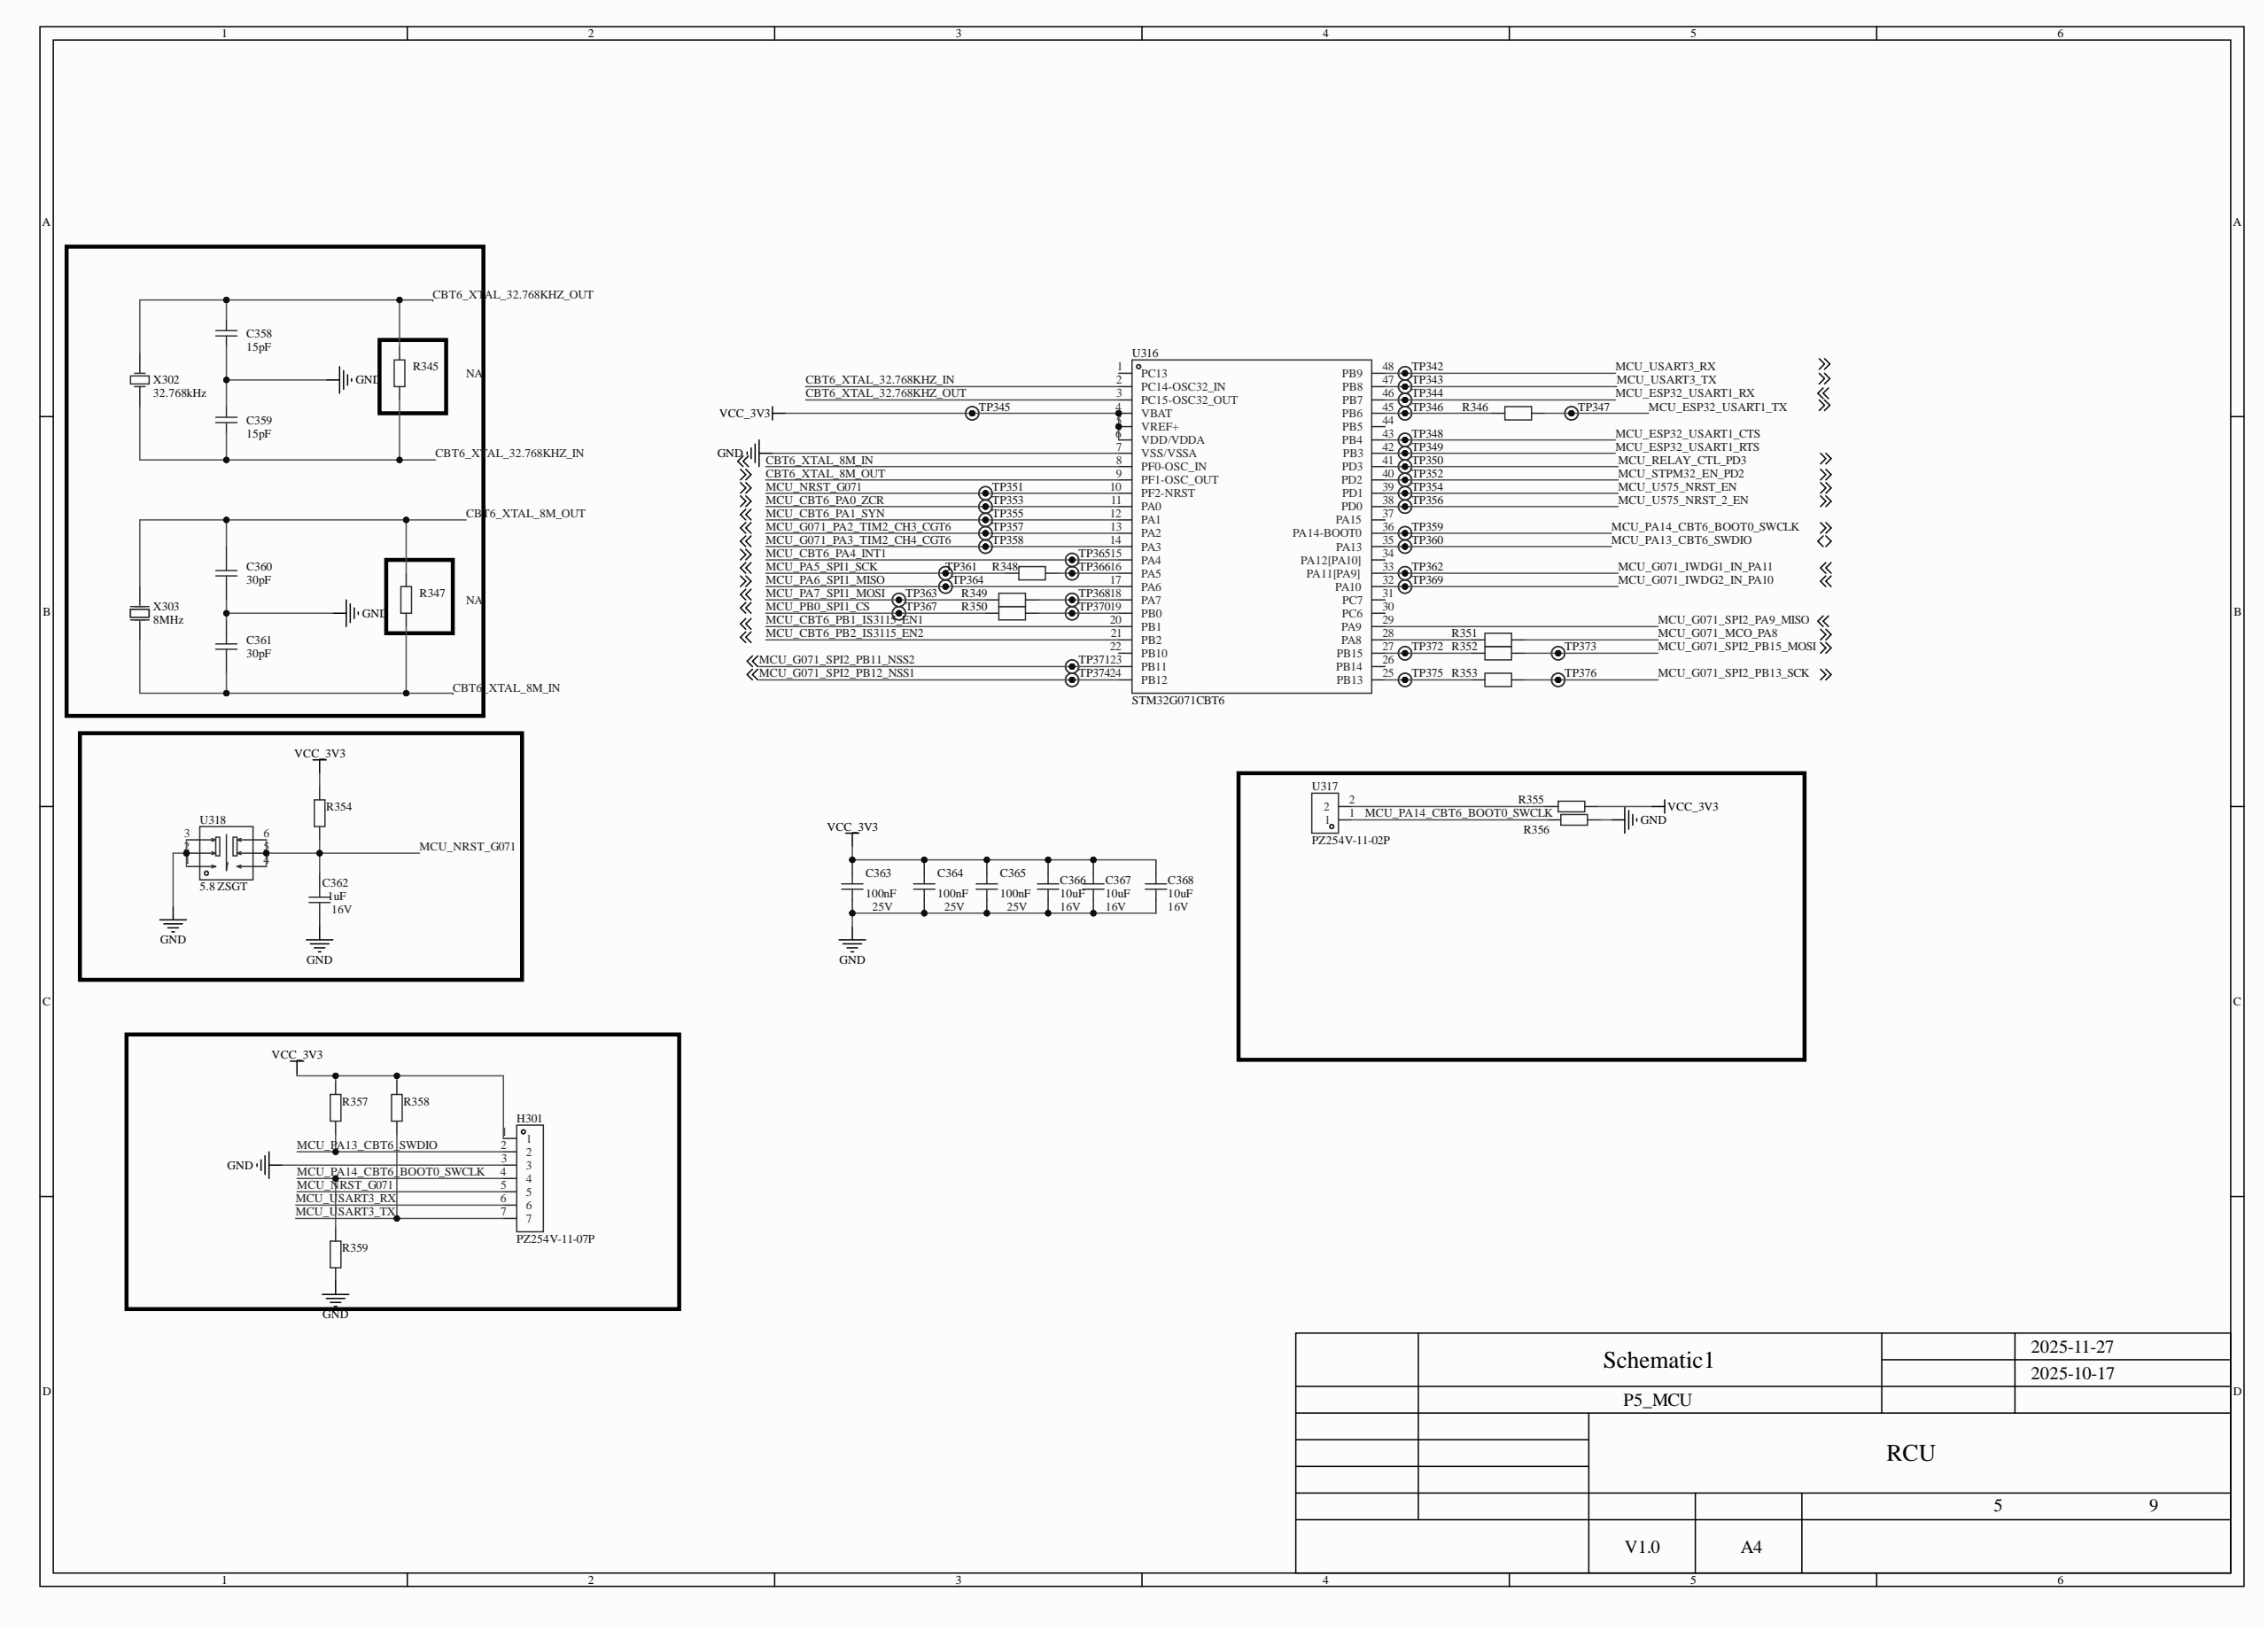Circuit board | Altium Designer | 424 parts | 202 nets | one sheet of the schematic
Parts on this sheet (reference | value | footprint):
C358 | 15pF | C0402
C359 | 15pF | C0402
C360 | 30pF | C0402
C361 | 30pF | C0402
C362 | 1uF | C0603
C363 | 100nF | C0603
C364 | 100nF | C0603
C365 | 100nF | C0603
C366 | 10uF | C0805
C367 | 10uF | C0805
C368 | 10uF | C0805
H301 | PZ254V-11-07P | HDR-TH_7P-P2.54-V-M
R345 | R0402
R346 | R0603
R347 | R0402
R348 | R0603
R349 | R0603
R350 | R0603
R351 | R0603
R352 | R0603
R353 | R0603
R354 | R0603
R355 | R0603
R356 | R0603
R357 | R0603
R358 | R0603
R359 | R0603
TP342 | Test-Point-0.5mm
TP343 | Test-Point-0.5mm
TP344 | Test-Point-0.5mm
TP345 | Test-Point-0.5mm
TP346 | Test-Point-0.5mm
TP347 | Test-Point-0.5mm
TP348 | Test-Point-0.5mm
TP349 | Test-Point-0.5mm
TP350 | Test-Point-0.5mm
TP351 | Test-Point-0.5mm
TP352 | Test-Point-0.5mm
TP353 | Test-Point-0.5mm
TP354 | Test-Point-0.5mm
TP355 | Test-Point-0.5mm
TP356 | Test-Point-0.5mm
TP357 | Test-Point-0.5mm
TP358 | Test-Point-0.5mm
TP359 | Test-Point-0.5mm
TP360 | Test-Point-0.5mm
TP361 | Test-Point-0.5mm
TP362 | Test-Point-0.5mm
TP363 | Test-Point-0.5mm
TP364 | Test-Point-0.5mm
TP365 | Test-Point-0.5mm
TP366 | Test-Point-0.5mm
TP367 | Test-Point-0.5mm
TP368 | Test-Point-0.5mm
TP369 | Test-Point-0.5mm
TP370 | Test-Point-0.5mm
TP371 | Test-Point-0.5mm
TP372 | Test-Point-0.5mm
TP373 | Test-Point-0.5mm
TP374 | Test-Point-0.5mm
TP375 | Test-Point-0.5mm
TP376 | Test-Point-0.5mm
U316 | STM32G071CBT6 | LQFP-48_L7.0-W7.0-P0.50-LS9.0-BL
U317 | PZ254V-11-02P | HDR-TH_2P-P2.54-V-M
U318 | 5.8 ZSGT | SW-TH_5.8ZSGT
X302 | 32.768kHz | OSC-TH_BD3.1-P0.8-D0.3
X303 | 8MHz | CRYSTAL-SMD_L5.0-W3.2
Nets of these parts (net: part-pin ...):
VCC_3V3: C363-1 C364-1 C365-1 C366-2 C367-2 C368-2 H301-1 R354-2 R355-2 R357-2 R358-2 TP345-1 U316-4 U316-5 U316-6
NetR355_1: R355-1 U317-2
NetR353_2: R353-2 TP375-1 U316-25
NetR352_2: R352-2 TP372-1 U316-27
NetR351_2: R351-2 U316-28
NetR350_1: R350-1 TP370-1 U316-19
NetR349_1: R349-1 TP368-1 U316-18
NetR348_1: R348-1 TP366-1 U316-16
NetR346_2: R346-2 TP346-1 U316-45
MCU_USART3_TX: H301-7 R358-1 TP343-1 U316-47
MCU_USART3_RX: H301-6 TP342-1 U316-48
MCU_U575_NRST_EN: TP354-1 U316-39
MCU_U575_NRST_2_EN: TP356-1 U316-38
MCU_STPM32_EN_PD2: TP352-1 U316-40
MCU_RELAY_CTL_PD3: TP350-1 U316-41
MCU_PB0_SPI1_CS: R350-2 TP367-1
MCU_PA14_CBT6_BOOT0_SWCLK: H301-4 R356-1 R359-1 TP359-1 U317-1 U316-36
MCU_PA13_CBT6_SWDIO: H301-2 R357-1 TP360-1 U316-35
MCU_PA7_SPI1_MOSI: R349-2 TP363-1
MCU_PA6_SPI1_MISO: TP364-1 U316-17
MCU_PA5_SPI1_SCK: R348-2 TP361-1
MCU_NRST_G071: C362-2 H301-5 R354-1 TP351-1 U318-4 U318-5 U318-6 U316-10
MCU_G071_SPI2_PB15_MOSI: R352-1 TP373-1
MCU_G071_SPI2_PB13_SCK: R353-1 TP376-1
MCU_G071_SPI2_PB12_NSS1: TP374-1 U316-24
MCU_G071_SPI2_PB11_NSS2: TP371-1 U316-23
MCU_G071_SPI2_PA9_MISO: U316-29
MCU_G071_PA3_TIM2_CH4_CGT6: TP358-1 U316-14
MCU_G071_PA2_TIM2_CH3_CGT6: TP357-1 U316-13
MCU_G071_MCO_PA8: R351-1
MCU_G071_IWDG2_IN_PA10: TP369-1 U316-32
MCU_G071_IWDG1_IN_PA11: TP362-1 U316-33
MCU_ESP32_USART1_TX: R346-1 TP347-1
MCU_ESP32_USART1_RX: TP344-1 U316-46
MCU_ESP32_USART1_RTS: TP349-1 U316-42
MCU_ESP32_USART1_CTS: TP348-1 U316-43
MCU_CBT6_PB2_IS3115_EN2: U316-21
MCU_CBT6_PB1_IS3115_EN1: U316-20
MCU_CBT6_PA4_INT1: TP365-1 U316-15
MCU_CBT6_PA1_SYN: TP355-1 U316-12
MCU_CBT6_PA0_ZCR: TP353-1 U316-11
GND: C358-1 C359-2 C360-2 C361-1 C362-1 C363-2 C364-2 C365-2 C366-1 C367-1 C368-1 H301-3 R356-2 R359-2 U318-1 U318-2 U318-3 U316-7
CBT6_XTAL_32.768KHZ_OUT: C358-2 R345-2 X302-2 U316-3
CBT6_XTAL_32.768KHZ_IN: C359-1 R345-1 X302-1 U316-2
CBT6_XTAL_8M_OUT: C360-1 R347-2 X303-2 U316-9
CBT6_XTAL_8M_IN: C361-2 R347-1 X303-1 U316-8